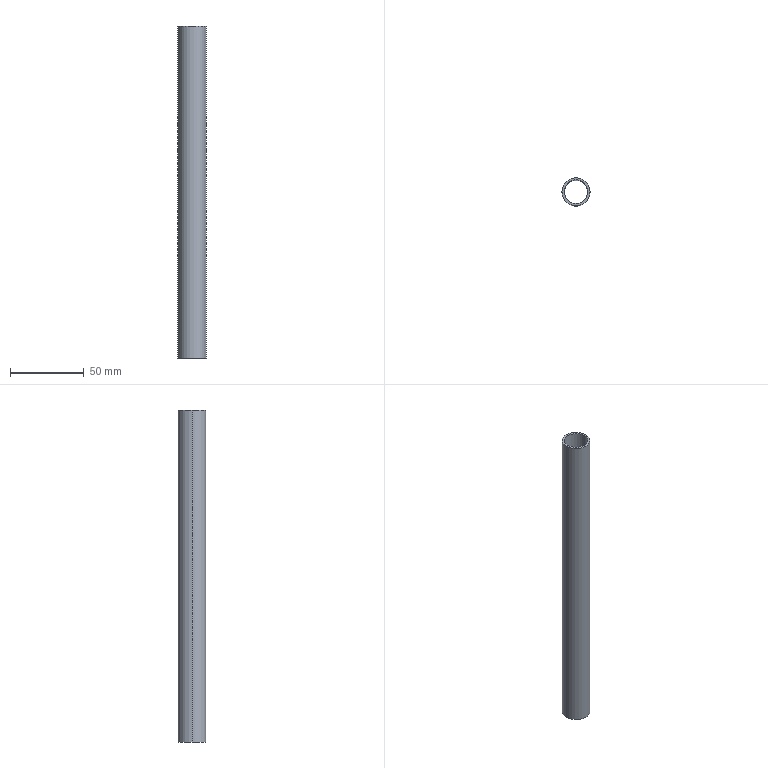Part | SolidWorks | features BaseBody 1 | 1 solid | 6 faces | box 19 x 19 x 225 mm | volume 18555 mm3 | cylinder 4 | plane 2 | commonest cylinder face diameters 16 x2 19 x2
STEP:
#1=CARTESIAN_POINT('',(-9.5,0.,112.5));
#2=VERTEX_POINT('',#1);
#3=CARTESIAN_POINT('',(9.5,0.,112.5));
#4=VERTEX_POINT('',#3);
#5=CARTESIAN_POINT('',(0.,0.,112.5));
#6=DIRECTION('',(0.,0.,-1.));
#7=DIRECTION('',(-1.,0.,0.));
#8=AXIS2_PLACEMENT_3D('',#5,#6,#7);
#9=CIRCLE('',#8,9.5);
#10=EDGE_CURVE('',#2,#4,#9,.T.);
#11=ORIENTED_EDGE('',*,*,#10,.T.);
#12=CARTESIAN_POINT('',(9.5,0.,-112.5));
#13=VERTEX_POINT('',#12);
#14=CARTESIAN_POINT('',(9.5,0.,112.5));
#15=DIRECTION('',(0.,0.,-1.));
#16=VECTOR('',#15,1000.);
#17=LINE('',#14,#16);
#18=EDGE_CURVE('',#4,#13,#17,.T.);
#19=ORIENTED_EDGE('',*,*,#18,.T.);
#20=CARTESIAN_POINT('',(-9.5,0.,-112.5));
#21=VERTEX_POINT('',#20);
#22=CARTESIAN_POINT('',(0.,0.,-112.5));
#23=DIRECTION('',(0.,0.,1.));
#24=DIRECTION('',(-1.,0.,0.));
#25=AXIS2_PLACEMENT_3D('',#22,#23,#24);
#26=CIRCLE('',#25,9.5);
#27=EDGE_CURVE('',#13,#21,#26,.T.);
#28=ORIENTED_EDGE('',*,*,#27,.T.);
#29=CARTESIAN_POINT('',(-9.5,0.,112.5));
#30=DIRECTION('',(0.,0.,-1.));
#31=VECTOR('',#30,1000.);
#32=LINE('',#29,#31);
#33=EDGE_CURVE('',#2,#21,#32,.T.);
#34=ORIENTED_EDGE('',*,*,#33,.F.);
#35=EDGE_LOOP('',(#11,#19,#28,#34));
#36=FACE_OUTER_BOUND('',#35,.T.);
#37=CARTESIAN_POINT('',(0.,0.,112.5));
#38=DIRECTION('',(0.,0.,-1.));
#39=DIRECTION('',(-1.,0.,0.));
#40=AXIS2_PLACEMENT_3D('',#37,#38,#39);
#41=CYLINDRICAL_SURFACE('',#40,9.5);
#42=ADVANCED_FACE('',(#36),#41,.T.);
#43=CARTESIAN_POINT('',(8.,0.,112.5));
#44=VERTEX_POINT('',#43);
#45=CARTESIAN_POINT('',(-8.,0.,112.5));
#46=VERTEX_POINT('',#45);
#47=CARTESIAN_POINT('',(0.,0.,112.5));
#48=DIRECTION('',(0.,0.,-1.));
#49=DIRECTION('',(-1.,0.,0.));
#50=AXIS2_PLACEMENT_3D('',#47,#48,#49);
#51=CIRCLE('',#50,8.);
#52=EDGE_CURVE('',#44,#46,#51,.T.);
#53=ORIENTED_EDGE('',*,*,#52,.F.);
#54=CARTESIAN_POINT('',(8.,0.,-112.5));
#55=VERTEX_POINT('',#54);
#56=CARTESIAN_POINT('',(8.,0.,112.5));
#57=DIRECTION('',(0.,0.,-1.));
#58=VECTOR('',#57,1000.);
#59=LINE('',#56,#58);
#60=EDGE_CURVE('',#44,#55,#59,.T.);
#61=ORIENTED_EDGE('',*,*,#60,.T.);
#62=CARTESIAN_POINT('',(-8.,0.,-112.5));
#63=VERTEX_POINT('',#62);
#64=CARTESIAN_POINT('',(0.,0.,-112.5));
#65=DIRECTION('',(0.,0.,-1.));
#66=DIRECTION('',(-1.,0.,0.));
#67=AXIS2_PLACEMENT_3D('',#64,#65,#66);
#68=CIRCLE('',#67,8.);
#69=EDGE_CURVE('',#55,#63,#68,.T.);
#70=ORIENTED_EDGE('',*,*,#69,.T.);
#71=CARTESIAN_POINT('',(-8.,0.,112.5));
#72=DIRECTION('',(0.,0.,-1.));
#73=VECTOR('',#72,1000.);
#74=LINE('',#71,#73);
#75=EDGE_CURVE('',#46,#63,#74,.T.);
#76=ORIENTED_EDGE('',*,*,#75,.F.);
#77=EDGE_LOOP('',(#53,#61,#70,#76));
#78=FACE_OUTER_BOUND('',#77,.T.);
#79=CARTESIAN_POINT('',(0.,0.,112.5));
#80=DIRECTION('',(0.,0.,-1.));
#81=DIRECTION('',(-1.,0.,0.));
#82=AXIS2_PLACEMENT_3D('',#79,#80,#81);
#83=CYLINDRICAL_SURFACE('',#82,8.);
#84=ADVANCED_FACE('',(#78),#83,.F.);
#85=ORIENTED_EDGE('',*,*,#18,.F.);
#86=CARTESIAN_POINT('',(0.,0.,112.5));
#87=DIRECTION('',(0.,0.,-1.));
#88=DIRECTION('',(-1.,0.,0.));
#89=AXIS2_PLACEMENT_3D('',#86,#87,#88);
#90=CIRCLE('',#89,9.5);
#91=EDGE_CURVE('',#4,#2,#90,.T.);
#92=ORIENTED_EDGE('',*,*,#91,.T.);
#93=ORIENTED_EDGE('',*,*,#33,.T.);
#94=CARTESIAN_POINT('',(0.,0.,-112.5));
#95=DIRECTION('',(0.,0.,1.));
#96=DIRECTION('',(-1.,0.,0.));
#97=AXIS2_PLACEMENT_3D('',#94,#95,#96);
#98=CIRCLE('',#97,9.5);
#99=EDGE_CURVE('',#21,#13,#98,.T.);
#100=ORIENTED_EDGE('',*,*,#99,.T.);
#101=EDGE_LOOP('',(#85,#92,#93,#100));
#102=FACE_OUTER_BOUND('',#101,.T.);
#103=CARTESIAN_POINT('',(0.,0.,112.5));
#104=DIRECTION('',(0.,0.,-1.));
#105=DIRECTION('',(-1.,0.,0.));
#106=AXIS2_PLACEMENT_3D('',#103,#104,#105);
#107=CYLINDRICAL_SURFACE('',#106,9.5);
#108=ADVANCED_FACE('',(#102),#107,.T.);
#109=CARTESIAN_POINT('',(0.,0.,-112.5));
#110=DIRECTION('',(0.,0.,-1.));
#111=DIRECTION('',(-1.,0.,0.));
#112=AXIS2_PLACEMENT_3D('',#109,#110,#111);
#113=CIRCLE('',#112,8.);
#114=EDGE_CURVE('',#63,#55,#113,.T.);
#115=ORIENTED_EDGE('',*,*,#114,.F.);
#116=ORIENTED_EDGE('',*,*,#69,.F.);
#117=EDGE_LOOP('',(#115,#116));
#118=FACE_BOUND('',#117,.T.);
#119=ORIENTED_EDGE('',*,*,#99,.F.);
#120=ORIENTED_EDGE('',*,*,#27,.F.);
#121=EDGE_LOOP('',(#119,#120));
#122=FACE_OUTER_BOUND('',#121,.T.);
#123=CARTESIAN_POINT('',(0.,0.,-112.5));
#124=DIRECTION('',(0.,0.,1.));
#125=DIRECTION('',(1.,0.,0.));
#126=AXIS2_PLACEMENT_3D('',#123,#124,#125);
#127=PLANE('',#126);
#128=ADVANCED_FACE('',(#118,#122),#127,.F.);
#129=CARTESIAN_POINT('',(0.,0.,112.5));
#130=DIRECTION('',(0.,0.,-1.));
#131=DIRECTION('',(-1.,0.,0.));
#132=AXIS2_PLACEMENT_3D('',#129,#130,#131);
#133=CIRCLE('',#132,8.);
#134=EDGE_CURVE('',#46,#44,#133,.T.);
#135=ORIENTED_EDGE('',*,*,#134,.T.);
#136=ORIENTED_EDGE('',*,*,#52,.T.);
#137=EDGE_LOOP('',(#135,#136));
#138=FACE_BOUND('',#137,.T.);
#139=ORIENTED_EDGE('',*,*,#10,.F.);
#140=ORIENTED_EDGE('',*,*,#91,.F.);
#141=EDGE_LOOP('',(#139,#140));
#142=FACE_OUTER_BOUND('',#141,.T.);
#143=CARTESIAN_POINT('',(0.,0.,112.5));
#144=DIRECTION('',(0.,0.,1.));
#145=DIRECTION('',(1.,0.,0.));
#146=AXIS2_PLACEMENT_3D('',#143,#144,#145);
#147=PLANE('',#146);
#148=ADVANCED_FACE('',(#138,#142),#147,.T.);
#149=ORIENTED_EDGE('',*,*,#60,.F.);
#150=ORIENTED_EDGE('',*,*,#134,.F.);
#151=ORIENTED_EDGE('',*,*,#75,.T.);
#152=ORIENTED_EDGE('',*,*,#114,.T.);
#153=EDGE_LOOP('',(#149,#150,#151,#152));
#154=FACE_OUTER_BOUND('',#153,.T.);
#155=CARTESIAN_POINT('',(0.,0.,112.5));
#156=DIRECTION('',(0.,0.,-1.));
#157=DIRECTION('',(-1.,0.,0.));
#158=AXIS2_PLACEMENT_3D('',#155,#156,#157);
#159=CYLINDRICAL_SURFACE('',#158,8.);
#160=ADVANCED_FACE('',(#154),#159,.F.);
#161=CLOSED_SHELL('',(#42,#84,#108,#128,#148,#160));
#162=MANIFOLD_SOLID_BREP('',#161);
#163=CARTESIAN_POINT('',(0.,0.,0.));
#164=DIRECTION('',(0.,0.,1.));
#165=DIRECTION('',(1.,0.,0.));
#166=AXIS2_PLACEMENT_3D('',#163,#164,#165);
#167=(LENGTH_UNIT()NAMED_UNIT(*)SI_UNIT(.MILLI.,.METRE.));
#168=UNCERTAINTY_MEASURE_WITH_UNIT(LENGTH_MEASURE(0.00001),#167,'','');
#169=(NAMED_UNIT(*)PLANE_ANGLE_UNIT()SI_UNIT($,.RADIAN.));
#170=(NAMED_UNIT(*)SI_UNIT($,.STERADIAN.)SOLID_ANGLE_UNIT());
#171=(GEOMETRIC_REPRESENTATION_CONTEXT(3)GLOBAL_UNCERTAINTY_ASSIGNED_CONTEXT((#168))GLOBAL_UNIT_ASSIGNED_CONTEXT((#167,#169,#170))REPRESENTATION_CONTEXT('',''));
#172=ADVANCED_BREP_SHAPE_REPRESENTATION('',(#162,#166),#171);